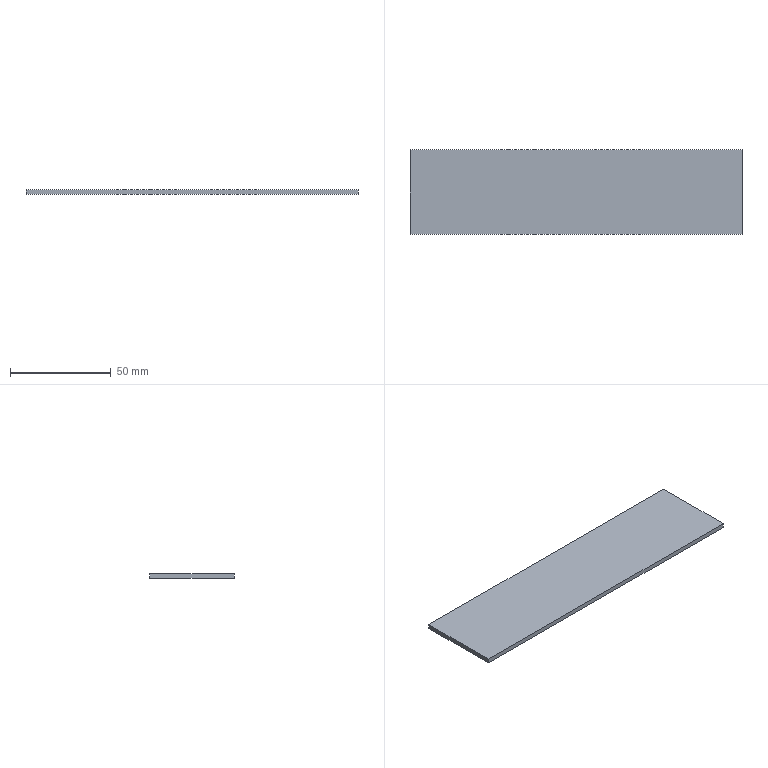Part | SolidWorks | features FlatPattern 1, SMBaseFlange 1, SheetMetal 1 | 1 solid | 6 faces | box 165 x 42 x 2.3 mm | volume 15939 mm3 | plane 6
STEP:
#1=CARTESIAN_POINT('',(0.,0.,0.));
#2=VERTEX_POINT('',#1);
#3=CARTESIAN_POINT('',(0.,-42.,0.));
#4=VERTEX_POINT('',#3);
#5=CARTESIAN_POINT('',(0.,0.,0.));
#6=DIRECTION('',(0.,-1.,0.));
#7=VECTOR('',#6,1000.);
#8=LINE('',#5,#7);
#9=EDGE_CURVE('',#2,#4,#8,.T.);
#10=ORIENTED_EDGE('',*,*,#9,.F.);
#11=CARTESIAN_POINT('',(0.,0.,-2.3));
#12=VERTEX_POINT('',#11);
#13=CARTESIAN_POINT('',(0.,0.,-2.3));
#14=DIRECTION('',(0.,0.,1.));
#15=VECTOR('',#14,1000.);
#16=LINE('',#13,#15);
#17=EDGE_CURVE('',#12,#2,#16,.T.);
#18=ORIENTED_EDGE('',*,*,#17,.F.);
#19=CARTESIAN_POINT('',(0.,-42.,-2.3));
#20=VERTEX_POINT('',#19);
#21=CARTESIAN_POINT('',(0.,0.,-2.3));
#22=DIRECTION('',(0.,-1.,0.));
#23=VECTOR('',#22,1000.);
#24=LINE('',#21,#23);
#25=EDGE_CURVE('',#12,#20,#24,.T.);
#26=ORIENTED_EDGE('',*,*,#25,.T.);
#27=CARTESIAN_POINT('',(0.,-42.,-2.3));
#28=DIRECTION('',(0.,0.,1.));
#29=VECTOR('',#28,1000.);
#30=LINE('',#27,#29);
#31=EDGE_CURVE('',#20,#4,#30,.T.);
#32=ORIENTED_EDGE('',*,*,#31,.T.);
#33=EDGE_LOOP('',(#10,#18,#26,#32));
#34=FACE_OUTER_BOUND('',#33,.T.);
#35=CARTESIAN_POINT('',(0.,0.,-2.3));
#36=DIRECTION('',(-1.,0.,0.));
#37=DIRECTION('',(0.,-1.,0.));
#38=AXIS2_PLACEMENT_3D('',#35,#36,#37);
#39=PLANE('',#38);
#40=ADVANCED_FACE('',(#34),#39,.T.);
#41=CARTESIAN_POINT('',(165.,0.,0.));
#42=VERTEX_POINT('',#41);
#43=CARTESIAN_POINT('',(0.,0.,0.));
#44=DIRECTION('',(-1.,0.,0.));
#45=VECTOR('',#44,1000.);
#46=LINE('',#43,#45);
#47=EDGE_CURVE('',#42,#2,#46,.T.);
#48=ORIENTED_EDGE('',*,*,#47,.F.);
#49=CARTESIAN_POINT('',(165.,0.,-2.3));
#50=VERTEX_POINT('',#49);
#51=CARTESIAN_POINT('',(165.,0.,-2.3));
#52=DIRECTION('',(0.,0.,1.));
#53=VECTOR('',#52,1000.);
#54=LINE('',#51,#53);
#55=EDGE_CURVE('',#50,#42,#54,.T.);
#56=ORIENTED_EDGE('',*,*,#55,.F.);
#57=CARTESIAN_POINT('',(0.,0.,-2.3));
#58=DIRECTION('',(-1.,0.,0.));
#59=VECTOR('',#58,1000.);
#60=LINE('',#57,#59);
#61=EDGE_CURVE('',#50,#12,#60,.T.);
#62=ORIENTED_EDGE('',*,*,#61,.T.);
#63=ORIENTED_EDGE('',*,*,#17,.T.);
#64=EDGE_LOOP('',(#48,#56,#62,#63));
#65=FACE_OUTER_BOUND('',#64,.T.);
#66=CARTESIAN_POINT('',(0.,0.,-2.3));
#67=DIRECTION('',(0.,1.,0.));
#68=DIRECTION('',(0.,0.,1.));
#69=AXIS2_PLACEMENT_3D('',#66,#67,#68);
#70=PLANE('',#69);
#71=ADVANCED_FACE('',(#65),#70,.T.);
#72=CARTESIAN_POINT('',(165.,-42.,0.));
#73=VERTEX_POINT('',#72);
#74=CARTESIAN_POINT('',(165.,0.,0.));
#75=DIRECTION('',(0.,1.,0.));
#76=VECTOR('',#75,1000.);
#77=LINE('',#74,#76);
#78=EDGE_CURVE('',#73,#42,#77,.T.);
#79=ORIENTED_EDGE('',*,*,#78,.F.);
#80=CARTESIAN_POINT('',(165.,-42.,-2.3));
#81=VERTEX_POINT('',#80);
#82=CARTESIAN_POINT('',(165.,-42.,-2.3));
#83=DIRECTION('',(0.,0.,1.));
#84=VECTOR('',#83,1000.);
#85=LINE('',#82,#84);
#86=EDGE_CURVE('',#81,#73,#85,.T.);
#87=ORIENTED_EDGE('',*,*,#86,.F.);
#88=CARTESIAN_POINT('',(165.,0.,-2.3));
#89=DIRECTION('',(0.,1.,0.));
#90=VECTOR('',#89,1000.);
#91=LINE('',#88,#90);
#92=EDGE_CURVE('',#81,#50,#91,.T.);
#93=ORIENTED_EDGE('',*,*,#92,.T.);
#94=ORIENTED_EDGE('',*,*,#55,.T.);
#95=EDGE_LOOP('',(#79,#87,#93,#94));
#96=FACE_OUTER_BOUND('',#95,.T.);
#97=CARTESIAN_POINT('',(165.,0.,-2.3));
#98=DIRECTION('',(1.,0.,0.));
#99=DIRECTION('',(0.,0.,-1.));
#100=AXIS2_PLACEMENT_3D('',#97,#98,#99);
#101=PLANE('',#100);
#102=ADVANCED_FACE('',(#96),#101,.T.);
#103=CARTESIAN_POINT('',(0.,-42.,0.));
#104=DIRECTION('',(1.,0.,0.));
#105=VECTOR('',#104,1000.);
#106=LINE('',#103,#105);
#107=EDGE_CURVE('',#4,#73,#106,.T.);
#108=ORIENTED_EDGE('',*,*,#107,.F.);
#109=ORIENTED_EDGE('',*,*,#31,.F.);
#110=CARTESIAN_POINT('',(0.,-42.,-2.3));
#111=DIRECTION('',(1.,0.,0.));
#112=VECTOR('',#111,1000.);
#113=LINE('',#110,#112);
#114=EDGE_CURVE('',#20,#81,#113,.T.);
#115=ORIENTED_EDGE('',*,*,#114,.T.);
#116=ORIENTED_EDGE('',*,*,#86,.T.);
#117=EDGE_LOOP('',(#108,#109,#115,#116));
#118=FACE_OUTER_BOUND('',#117,.T.);
#119=CARTESIAN_POINT('',(0.,-42.,-2.3));
#120=DIRECTION('',(0.,-1.,0.));
#121=DIRECTION('',(0.,0.,-1.));
#122=AXIS2_PLACEMENT_3D('',#119,#120,#121);
#123=PLANE('',#122);
#124=ADVANCED_FACE('',(#118),#123,.T.);
#125=ORIENTED_EDGE('',*,*,#25,.F.);
#126=ORIENTED_EDGE('',*,*,#61,.F.);
#127=ORIENTED_EDGE('',*,*,#92,.F.);
#128=ORIENTED_EDGE('',*,*,#114,.F.);
#129=EDGE_LOOP('',(#125,#126,#127,#128));
#130=FACE_OUTER_BOUND('',#129,.T.);
#131=CARTESIAN_POINT('',(0.,0.,-2.3));
#132=DIRECTION('',(0.,0.,1.));
#133=DIRECTION('',(1.,0.,0.));
#134=AXIS2_PLACEMENT_3D('',#131,#132,#133);
#135=PLANE('',#134);
#136=ADVANCED_FACE('',(#130),#135,.F.);
#137=ORIENTED_EDGE('',*,*,#9,.T.);
#138=ORIENTED_EDGE('',*,*,#107,.T.);
#139=ORIENTED_EDGE('',*,*,#78,.T.);
#140=ORIENTED_EDGE('',*,*,#47,.T.);
#141=EDGE_LOOP('',(#137,#138,#139,#140));
#142=FACE_OUTER_BOUND('',#141,.T.);
#143=CARTESIAN_POINT('',(0.,0.,0.));
#144=DIRECTION('',(0.,0.,1.));
#145=DIRECTION('',(1.,0.,0.));
#146=AXIS2_PLACEMENT_3D('',#143,#144,#145);
#147=PLANE('',#146);
#148=ADVANCED_FACE('',(#142),#147,.T.);
#149=CLOSED_SHELL('',(#40,#71,#102,#124,#136,#148));
#150=MANIFOLD_SOLID_BREP('',#149);
#151=CARTESIAN_POINT('',(0.,0.,0.));
#152=DIRECTION('',(0.,0.,1.));
#153=DIRECTION('',(1.,0.,0.));
#154=AXIS2_PLACEMENT_3D('',#151,#152,#153);
#155=(LENGTH_UNIT()NAMED_UNIT(*)SI_UNIT(.MILLI.,.METRE.));
#156=UNCERTAINTY_MEASURE_WITH_UNIT(LENGTH_MEASURE(0.00001),#155,'','');
#157=(NAMED_UNIT(*)PLANE_ANGLE_UNIT()SI_UNIT($,.RADIAN.));
#158=(NAMED_UNIT(*)SI_UNIT($,.STERADIAN.)SOLID_ANGLE_UNIT());
#159=(GEOMETRIC_REPRESENTATION_CONTEXT(3)GLOBAL_UNCERTAINTY_ASSIGNED_CONTEXT((#156))GLOBAL_UNIT_ASSIGNED_CONTEXT((#155,#157,#158))REPRESENTATION_CONTEXT('',''));
#160=ADVANCED_BREP_SHAPE_REPRESENTATION('',(#150,#154),#159);